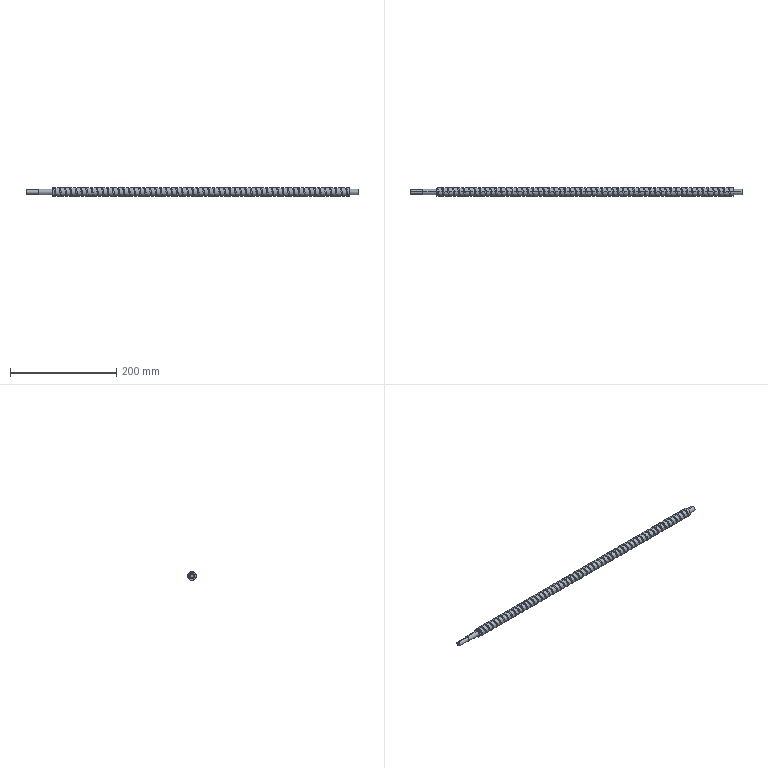Part | SolidWorks | features BaseBody 1 | 1 solid | 151 faces | box 626 x 16 x 16 mm | volume 109348 mm3 | cylinder 121 | spline 25 | plane 5 | commonest cylinder face diameters 16 x115 10 x4 8 x2